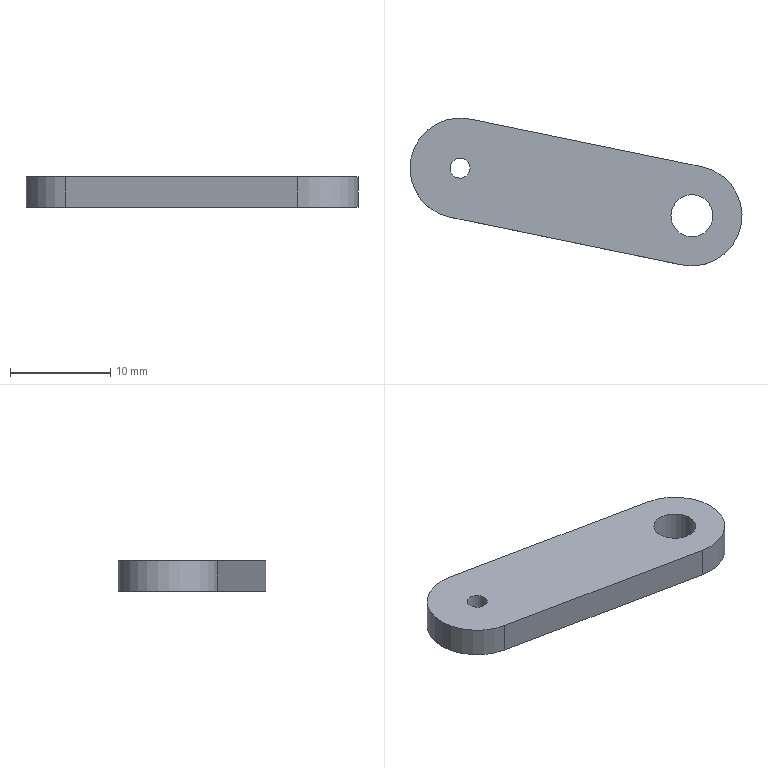Part | NX | features DATUM_CSYS 2, OFFSET_REGION 2, BREP 1, EXTRUDE 1, SCALE 1, SKETCH 1 | 1 solid | 8 faces | box 33.164 x 14.761 x 3 mm | volume 894.076 mm3 | cylinder 4 | plane 4 | commonest cylinder face diameters 10 x2 2 x1 4.2 x1
STEP:
#1=CARTESIAN_POINT('',(-17.528,-37.012,-12.5));
#2=VERTEX_POINT('',#1);
#3=CARTESIAN_POINT('',(-18.528,-37.012,-12.5));
#4=DIRECTION('',(0.,0.,1.));
#5=DIRECTION('',(1.,0.,0.));
#6=AXIS2_PLACEMENT_3D('',#3,#4,#5);
#7=CIRCLE('',#6,1.);
#8=EDGE_CURVE('',#2,#2,#7,.T.);
#9=ORIENTED_EDGE('',*,*,#8,.T.);
#10=EDGE_LOOP('',(#9));
#11=FACE_BOUND('',#10,.T.);
#12=CARTESIAN_POINT('',(-19.507,-36.81,-15.5));
#13=VERTEX_POINT('',#12);
#14=CARTESIAN_POINT('',(-18.528,-37.012,-15.5));
#15=DIRECTION('',(0.,0.,1.));
#16=DIRECTION('',(-0.9795,0.2013,0.));
#17=AXIS2_PLACEMENT_3D('',#14,#15,#16);
#18=CIRCLE('',#17,1.);
#19=EDGE_CURVE('',#13,#13,#18,.T.);
#20=ORIENTED_EDGE('',*,*,#19,.F.);
#21=EDGE_LOOP('',(#20));
#22=FACE_BOUND('',#21,.T.);
#23=CARTESIAN_POINT('',(-18.528,-37.012,-14.5));
#24=DIRECTION('',(0.,0.,1.));
#25=DIRECTION('',(-0.9795,0.2013,0.));
#26=AXIS2_PLACEMENT_3D('',#23,#24,#25);
#27=CYLINDRICAL_SURFACE('',#26,1.);
#28=ADVANCED_FACE('',(#11,#22),#27,.F.);
#29=CARTESIAN_POINT('',(3.629,-46.671,-12.5));
#30=VERTEX_POINT('',#29);
#31=CARTESIAN_POINT('',(5.643,-36.875,-12.5));
#32=VERTEX_POINT('',#31);
#33=CARTESIAN_POINT('',(4.636,-41.773,-12.5));
#34=DIRECTION('',(0.,0.,1.));
#35=DIRECTION('',(1.,0.,0.));
#36=AXIS2_PLACEMENT_3D('',#33,#34,#35);
#37=CIRCLE('',#36,5.);
#38=EDGE_CURVE('',#30,#32,#37,.T.);
#39=ORIENTED_EDGE('',*,*,#38,.F.);
#40=CARTESIAN_POINT('',(3.629,-46.671,-15.5));
#41=VERTEX_POINT('',#40);
#42=CARTESIAN_POINT('',(3.629,-46.671,-14.5));
#43=DIRECTION('',(0.,0.,-1.));
#44=VECTOR('',#43,1000.);
#45=LINE('',#42,#44);
#46=EDGE_CURVE('',#30,#41,#45,.T.);
#47=ORIENTED_EDGE('',*,*,#46,.T.);
#48=CARTESIAN_POINT('',(5.643,-36.875,-15.5));
#49=VERTEX_POINT('',#48);
#50=CARTESIAN_POINT('',(4.636,-41.773,-15.5));
#51=DIRECTION('',(0.,0.,1.));
#52=DIRECTION('',(1.,0.,0.));
#53=AXIS2_PLACEMENT_3D('',#50,#51,#52);
#54=CIRCLE('',#53,5.);
#55=EDGE_CURVE('',#41,#49,#54,.T.);
#56=ORIENTED_EDGE('',*,*,#55,.T.);
#57=CARTESIAN_POINT('',(5.643,-36.875,-14.5));
#58=DIRECTION('',(0.,0.,1.));
#59=VECTOR('',#58,1000.);
#60=LINE('',#57,#59);
#61=EDGE_CURVE('',#32,#49,#60,.F.);
#62=ORIENTED_EDGE('',*,*,#61,.F.);
#63=EDGE_LOOP('',(#39,#47,#56,#62));
#64=FACE_BOUND('',#63,.T.);
#65=CARTESIAN_POINT('',(4.636,-41.773,-14.5));
#66=DIRECTION('',(0.,0.,-1.));
#67=DIRECTION('',(0.9795,-0.2013,0.));
#68=AXIS2_PLACEMENT_3D('',#65,#66,#67);
#69=CYLINDRICAL_SURFACE('',#68,5.);
#70=ADVANCED_FACE('',(#64),#69,.T.);
#71=CARTESIAN_POINT('',(-17.521,-32.114,-15.5));
#72=VERTEX_POINT('',#71);
#73=CARTESIAN_POINT('',(5.643,-36.875,-15.5));
#74=DIRECTION('',(-0.9795,0.2013,0.));
#75=VECTOR('',#74,1000.);
#76=LINE('',#73,#75);
#77=EDGE_CURVE('',#49,#72,#76,.T.);
#78=ORIENTED_EDGE('',*,*,#77,.T.);
#79=CARTESIAN_POINT('',(-17.521,-32.114,-12.5));
#80=VERTEX_POINT('',#79);
#81=CARTESIAN_POINT('',(-17.521,-32.114,-14.5));
#82=DIRECTION('',(0.,0.,-1.));
#83=VECTOR('',#82,1000.);
#84=LINE('',#81,#83);
#85=EDGE_CURVE('',#80,#72,#84,.T.);
#86=ORIENTED_EDGE('',*,*,#85,.F.);
#87=CARTESIAN_POINT('',(5.643,-36.875,-12.5));
#88=DIRECTION('',(-0.9795,0.2013,0.));
#89=VECTOR('',#88,1000.);
#90=LINE('',#87,#89);
#91=EDGE_CURVE('',#32,#80,#90,.T.);
#92=ORIENTED_EDGE('',*,*,#91,.F.);
#93=ORIENTED_EDGE('',*,*,#61,.T.);
#94=EDGE_LOOP('',(#78,#86,#92,#93));
#95=FACE_BOUND('',#94,.T.);
#96=CARTESIAN_POINT('',(5.643,-36.875,-14.5));
#97=DIRECTION('',(-0.2013,-0.9795,0.));
#98=DIRECTION('',(0.9795,-0.2013,0.));
#99=AXIS2_PLACEMENT_3D('',#96,#97,#98);
#100=PLANE('',#99);
#101=ADVANCED_FACE('',(#95),#100,.F.);
#102=CARTESIAN_POINT('',(-19.535,-41.909,-15.5));
#103=VERTEX_POINT('',#102);
#104=CARTESIAN_POINT('',(-18.528,-37.012,-15.5));
#105=DIRECTION('',(0.,0.,1.));
#106=DIRECTION('',(1.,0.,0.));
#107=AXIS2_PLACEMENT_3D('',#104,#105,#106);
#108=CIRCLE('',#107,5.);
#109=EDGE_CURVE('',#72,#103,#108,.T.);
#110=ORIENTED_EDGE('',*,*,#109,.T.);
#111=CARTESIAN_POINT('',(-19.535,-41.909,-12.5));
#112=VERTEX_POINT('',#111);
#113=CARTESIAN_POINT('',(-19.535,-41.909,-14.5));
#114=DIRECTION('',(0.,0.,1.));
#115=VECTOR('',#114,1000.);
#116=LINE('',#113,#115);
#117=EDGE_CURVE('',#112,#103,#116,.F.);
#118=ORIENTED_EDGE('',*,*,#117,.F.);
#119=CARTESIAN_POINT('',(-18.528,-37.012,-12.5));
#120=DIRECTION('',(0.,0.,1.));
#121=DIRECTION('',(1.,0.,0.));
#122=AXIS2_PLACEMENT_3D('',#119,#120,#121);
#123=CIRCLE('',#122,5.);
#124=EDGE_CURVE('',#80,#112,#123,.T.);
#125=ORIENTED_EDGE('',*,*,#124,.F.);
#126=ORIENTED_EDGE('',*,*,#85,.T.);
#127=EDGE_LOOP('',(#110,#118,#125,#126));
#128=FACE_BOUND('',#127,.T.);
#129=CARTESIAN_POINT('',(-18.528,-37.012,-14.5));
#130=DIRECTION('',(0.,0.,-1.));
#131=DIRECTION('',(0.9795,-0.2013,0.));
#132=AXIS2_PLACEMENT_3D('',#129,#130,#131);
#133=CYLINDRICAL_SURFACE('',#132,5.);
#134=ADVANCED_FACE('',(#128),#133,.T.);
#135=CARTESIAN_POINT('',(3.629,-46.671,-15.5));
#136=DIRECTION('',(0.9795,-0.2013,0.));
#137=VECTOR('',#136,1000.);
#138=LINE('',#135,#137);
#139=EDGE_CURVE('',#103,#41,#138,.T.);
#140=ORIENTED_EDGE('',*,*,#139,.T.);
#141=ORIENTED_EDGE('',*,*,#46,.F.);
#142=CARTESIAN_POINT('',(3.629,-46.671,-12.5));
#143=DIRECTION('',(0.9795,-0.2013,0.));
#144=VECTOR('',#143,1000.);
#145=LINE('',#142,#144);
#146=EDGE_CURVE('',#112,#30,#145,.T.);
#147=ORIENTED_EDGE('',*,*,#146,.F.);
#148=ORIENTED_EDGE('',*,*,#117,.T.);
#149=EDGE_LOOP('',(#140,#141,#147,#148));
#150=FACE_BOUND('',#149,.T.);
#151=CARTESIAN_POINT('',(3.629,-46.671,-14.5));
#152=DIRECTION('',(0.2013,0.9795,0.));
#153=DIRECTION('',(-0.9795,0.2013,0.));
#154=AXIS2_PLACEMENT_3D('',#151,#152,#153);
#155=PLANE('',#154);
#156=ADVANCED_FACE('',(#150),#155,.F.);
#157=CARTESIAN_POINT('',(6.736,-41.773,-12.5));
#158=VERTEX_POINT('',#157);
#159=CARTESIAN_POINT('',(4.636,-41.773,-12.5));
#160=DIRECTION('',(0.,0.,1.));
#161=DIRECTION('',(1.,0.,0.));
#162=AXIS2_PLACEMENT_3D('',#159,#160,#161);
#163=CIRCLE('',#162,2.1);
#164=EDGE_CURVE('',#158,#158,#163,.F.);
#165=ORIENTED_EDGE('',*,*,#164,.T.);
#166=EDGE_LOOP('',(#165));
#167=FACE_BOUND('',#166,.T.);
#168=ORIENTED_EDGE('',*,*,#8,.F.);
#169=EDGE_LOOP('',(#168));
#170=FACE_BOUND('',#169,.T.);
#171=ORIENTED_EDGE('',*,*,#146,.T.);
#172=ORIENTED_EDGE('',*,*,#38,.T.);
#173=ORIENTED_EDGE('',*,*,#91,.T.);
#174=ORIENTED_EDGE('',*,*,#124,.T.);
#175=EDGE_LOOP('',(#171,#172,#173,#174));
#176=FACE_BOUND('',#175,.T.);
#177=CARTESIAN_POINT('',(4.636,-41.773,-12.5));
#178=DIRECTION('',(0.,0.,1.));
#179=DIRECTION('',(-0.9795,0.2013,0.));
#180=AXIS2_PLACEMENT_3D('',#177,#178,#179);
#181=PLANE('',#180);
#182=ADVANCED_FACE('',(#167,#170,#176),#181,.T.);
#183=CARTESIAN_POINT('',(6.736,-41.773,-15.5));
#184=VERTEX_POINT('',#183);
#185=CARTESIAN_POINT('',(4.636,-41.773,-15.5));
#186=DIRECTION('',(0.,0.,1.));
#187=DIRECTION('',(1.,0.,0.));
#188=AXIS2_PLACEMENT_3D('',#185,#186,#187);
#189=CIRCLE('',#188,2.1);
#190=EDGE_CURVE('',#184,#184,#189,.F.);
#191=ORIENTED_EDGE('',*,*,#190,.F.);
#192=EDGE_LOOP('',(#191));
#193=FACE_BOUND('',#192,.T.);
#194=ORIENTED_EDGE('',*,*,#19,.T.);
#195=EDGE_LOOP('',(#194));
#196=FACE_BOUND('',#195,.T.);
#197=ORIENTED_EDGE('',*,*,#55,.F.);
#198=ORIENTED_EDGE('',*,*,#139,.F.);
#199=ORIENTED_EDGE('',*,*,#109,.F.);
#200=ORIENTED_EDGE('',*,*,#77,.F.);
#201=EDGE_LOOP('',(#197,#198,#199,#200));
#202=FACE_BOUND('',#201,.T.);
#203=CARTESIAN_POINT('',(4.636,-41.773,-15.5));
#204=DIRECTION('',(0.,0.,1.));
#205=DIRECTION('',(-0.9795,0.2013,0.));
#206=AXIS2_PLACEMENT_3D('',#203,#204,#205);
#207=PLANE('',#206);
#208=ADVANCED_FACE('',(#193,#196,#202),#207,.F.);
#209=ORIENTED_EDGE('',*,*,#164,.F.);
#210=EDGE_LOOP('',(#209));
#211=FACE_BOUND('',#210,.T.);
#212=ORIENTED_EDGE('',*,*,#190,.T.);
#213=EDGE_LOOP('',(#212));
#214=FACE_BOUND('',#213,.T.);
#215=CARTESIAN_POINT('',(4.636,-41.773,-9.5));
#216=DIRECTION('',(0.,0.,-1.));
#217=DIRECTION('',(-1.,0.,0.));
#218=AXIS2_PLACEMENT_3D('',#215,#216,#217);
#219=CYLINDRICAL_SURFACE('',#218,2.1);
#220=ADVANCED_FACE('',(#211,#214),#219,.F.);
#221=CLOSED_SHELL('',(#28,#70,#101,#134,#156,#182,#208,#220));
#222=MANIFOLD_SOLID_BREP('',#221);
#223=(LENGTH_UNIT()NAMED_UNIT(*)SI_UNIT(.MILLI.,.METRE.));
#224=UNCERTAINTY_MEASURE_WITH_UNIT(LENGTH_MEASURE(0.00001),#223,'','');
#225=(NAMED_UNIT(*)PLANE_ANGLE_UNIT()SI_UNIT($,.RADIAN.));
#226=(NAMED_UNIT(*)SI_UNIT($,.STERADIAN.)SOLID_ANGLE_UNIT());
#227=(GEOMETRIC_REPRESENTATION_CONTEXT(3)GLOBAL_UNCERTAINTY_ASSIGNED_CONTEXT((#224))GLOBAL_UNIT_ASSIGNED_CONTEXT((#223,#225,#226))REPRESENTATION_CONTEXT('',''));
#228=ADVANCED_BREP_SHAPE_REPRESENTATION('',(#222),#227);